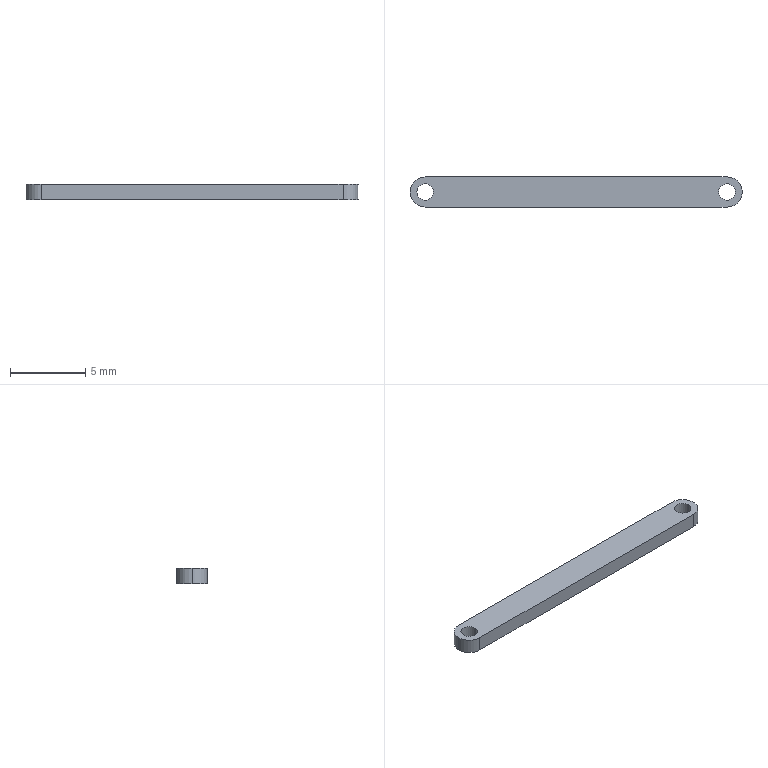Part | SolidWorks | features Extrusion 1, ICE 1 | 1 solid | 11 faces | box 22 x 2 x 1 mm | volume 41.241 mm3 | cylinder 7 | plane 4 | commonest cylinder face diameters 1.1 x4 2 x3
STEP:
#1=CARTESIAN_POINT('',(9.45,0.,0.5));
#2=VERTEX_POINT('',#1);
#3=CARTESIAN_POINT('',(10.55,0.,0.5));
#4=VERTEX_POINT('',#3);
#5=CARTESIAN_POINT('',(10.,0.,0.5));
#6=DIRECTION('',(0.,0.,1.));
#7=DIRECTION('',(1.,0.,0.));
#8=AXIS2_PLACEMENT_3D('',#5,#6,#7);
#9=CIRCLE('',#8,0.55);
#10=EDGE_CURVE('',#2,#4,#9,.T.);
#11=ORIENTED_EDGE('',*,*,#10,.T.);
#12=CARTESIAN_POINT('',(10.55,0.,-0.5));
#13=VERTEX_POINT('',#12);
#14=CARTESIAN_POINT('',(10.55,0.,0.5));
#15=DIRECTION('',(0.,0.,-1.));
#16=VECTOR('',#15,1000.);
#17=LINE('',#14,#16);
#18=EDGE_CURVE('',#4,#13,#17,.T.);
#19=ORIENTED_EDGE('',*,*,#18,.T.);
#20=CARTESIAN_POINT('',(9.45,0.,-0.5));
#21=VERTEX_POINT('',#20);
#22=CARTESIAN_POINT('',(10.,0.,-0.5));
#23=DIRECTION('',(0.,0.,1.));
#24=DIRECTION('',(1.,0.,0.));
#25=AXIS2_PLACEMENT_3D('',#22,#23,#24);
#26=CIRCLE('',#25,0.55);
#27=EDGE_CURVE('',#21,#13,#26,.T.);
#28=ORIENTED_EDGE('',*,*,#27,.F.);
#29=CARTESIAN_POINT('',(9.45,0.,0.5));
#30=DIRECTION('',(0.,0.,-1.));
#31=VECTOR('',#30,1000.);
#32=LINE('',#29,#31);
#33=EDGE_CURVE('',#2,#21,#32,.T.);
#34=ORIENTED_EDGE('',*,*,#33,.F.);
#35=EDGE_LOOP('',(#11,#19,#28,#34));
#36=FACE_OUTER_BOUND('',#35,.T.);
#37=CARTESIAN_POINT('',(10.,0.,0.5));
#38=DIRECTION('',(0.,0.,-1.));
#39=DIRECTION('',(-1.,0.,0.));
#40=AXIS2_PLACEMENT_3D('',#37,#38,#39);
#41=CYLINDRICAL_SURFACE('',#40,0.55);
#42=ADVANCED_FACE('',(#36),#41,.F.);
#43=CARTESIAN_POINT('',(-10.55,0.,0.5));
#44=VERTEX_POINT('',#43);
#45=CARTESIAN_POINT('',(-9.45,0.,0.5));
#46=VERTEX_POINT('',#45);
#47=CARTESIAN_POINT('',(-10.,0.,0.5));
#48=DIRECTION('',(0.,0.,1.));
#49=DIRECTION('',(1.,0.,0.));
#50=AXIS2_PLACEMENT_3D('',#47,#48,#49);
#51=CIRCLE('',#50,0.55);
#52=EDGE_CURVE('',#44,#46,#51,.T.);
#53=ORIENTED_EDGE('',*,*,#52,.T.);
#54=CARTESIAN_POINT('',(-9.45,0.,-0.5));
#55=VERTEX_POINT('',#54);
#56=CARTESIAN_POINT('',(-9.45,0.,0.5));
#57=DIRECTION('',(0.,0.,-1.));
#58=VECTOR('',#57,1000.);
#59=LINE('',#56,#58);
#60=EDGE_CURVE('',#46,#55,#59,.T.);
#61=ORIENTED_EDGE('',*,*,#60,.T.);
#62=CARTESIAN_POINT('',(-10.55,0.,-0.5));
#63=VERTEX_POINT('',#62);
#64=CARTESIAN_POINT('',(-10.,0.,-0.5));
#65=DIRECTION('',(0.,0.,1.));
#66=DIRECTION('',(1.,0.,0.));
#67=AXIS2_PLACEMENT_3D('',#64,#65,#66);
#68=CIRCLE('',#67,0.55);
#69=EDGE_CURVE('',#63,#55,#68,.T.);
#70=ORIENTED_EDGE('',*,*,#69,.F.);
#71=CARTESIAN_POINT('',(-10.55,0.,0.5));
#72=DIRECTION('',(0.,0.,-1.));
#73=VECTOR('',#72,1000.);
#74=LINE('',#71,#73);
#75=EDGE_CURVE('',#44,#63,#74,.T.);
#76=ORIENTED_EDGE('',*,*,#75,.F.);
#77=EDGE_LOOP('',(#53,#61,#70,#76));
#78=FACE_OUTER_BOUND('',#77,.T.);
#79=CARTESIAN_POINT('',(-10.,0.,0.5));
#80=DIRECTION('',(0.,0.,-1.));
#81=DIRECTION('',(-1.,0.,0.));
#82=AXIS2_PLACEMENT_3D('',#79,#80,#81);
#83=CYLINDRICAL_SURFACE('',#82,0.55);
#84=ADVANCED_FACE('',(#78),#83,.F.);
#85=CARTESIAN_POINT('',(-11.,0.,0.5));
#86=VERTEX_POINT('',#85);
#87=CARTESIAN_POINT('',(-10.,-1.,0.5));
#88=VERTEX_POINT('',#87);
#89=CARTESIAN_POINT('',(-10.,0.,0.5));
#90=DIRECTION('',(0.,0.,1.));
#91=DIRECTION('',(1.,0.,0.));
#92=AXIS2_PLACEMENT_3D('',#89,#90,#91);
#93=CIRCLE('',#92,1.);
#94=EDGE_CURVE('',#86,#88,#93,.T.);
#95=ORIENTED_EDGE('',*,*,#94,.F.);
#96=CARTESIAN_POINT('',(-11.,0.,-0.5));
#97=VERTEX_POINT('',#96);
#98=CARTESIAN_POINT('',(-11.,0.,0.5));
#99=DIRECTION('',(0.,0.,-1.));
#100=VECTOR('',#99,1000.);
#101=LINE('',#98,#100);
#102=EDGE_CURVE('',#86,#97,#101,.T.);
#103=ORIENTED_EDGE('',*,*,#102,.T.);
#104=CARTESIAN_POINT('',(-10.,-1.,-0.5));
#105=VERTEX_POINT('',#104);
#106=CARTESIAN_POINT('',(-10.,0.,-0.5));
#107=DIRECTION('',(0.,0.,1.));
#108=DIRECTION('',(1.,0.,0.));
#109=AXIS2_PLACEMENT_3D('',#106,#107,#108);
#110=CIRCLE('',#109,1.);
#111=EDGE_CURVE('',#97,#105,#110,.T.);
#112=ORIENTED_EDGE('',*,*,#111,.T.);
#113=CARTESIAN_POINT('',(-10.,-1.,0.5));
#114=DIRECTION('',(0.,0.,-1.));
#115=VECTOR('',#114,1000.);
#116=LINE('',#113,#115);
#117=EDGE_CURVE('',#88,#105,#116,.T.);
#118=ORIENTED_EDGE('',*,*,#117,.F.);
#119=EDGE_LOOP('',(#95,#103,#112,#118));
#120=FACE_OUTER_BOUND('',#119,.T.);
#121=CARTESIAN_POINT('',(-10.,0.,0.5));
#122=DIRECTION('',(0.,0.,-1.));
#123=DIRECTION('',(-1.,0.,0.));
#124=AXIS2_PLACEMENT_3D('',#121,#122,#123);
#125=CYLINDRICAL_SURFACE('',#124,1.);
#126=ADVANCED_FACE('',(#120),#125,.T.);
#127=ORIENTED_EDGE('',*,*,#52,.F.);
#128=CARTESIAN_POINT('',(-10.,0.,0.5));
#129=DIRECTION('',(0.,0.,1.));
#130=DIRECTION('',(1.,0.,0.));
#131=AXIS2_PLACEMENT_3D('',#128,#129,#130);
#132=CIRCLE('',#131,0.55);
#133=EDGE_CURVE('',#46,#44,#132,.T.);
#134=ORIENTED_EDGE('',*,*,#133,.F.);
#135=EDGE_LOOP('',(#127,#134));
#136=FACE_BOUND('',#135,.T.);
#137=CARTESIAN_POINT('',(-10.,1.,0.5));
#138=VERTEX_POINT('',#137);
#139=CARTESIAN_POINT('',(-10.,0.,0.5));
#140=DIRECTION('',(0.,0.,1.));
#141=DIRECTION('',(1.,0.,0.));
#142=AXIS2_PLACEMENT_3D('',#139,#140,#141);
#143=CIRCLE('',#142,1.);
#144=EDGE_CURVE('',#138,#86,#143,.T.);
#145=ORIENTED_EDGE('',*,*,#144,.T.);
#146=ORIENTED_EDGE('',*,*,#94,.T.);
#147=CARTESIAN_POINT('',(10.,-1.,0.5));
#148=VERTEX_POINT('',#147);
#149=CARTESIAN_POINT('',(-10.,-1.,0.5));
#150=DIRECTION('',(1.,0.,0.));
#151=VECTOR('',#150,1000.);
#152=LINE('',#149,#151);
#153=EDGE_CURVE('',#88,#148,#152,.T.);
#154=ORIENTED_EDGE('',*,*,#153,.T.);
#155=CARTESIAN_POINT('',(10.,1.,0.5));
#156=VERTEX_POINT('',#155);
#157=CARTESIAN_POINT('',(10.,0.,0.5));
#158=DIRECTION('',(0.,0.,1.));
#159=DIRECTION('',(1.,0.,0.));
#160=AXIS2_PLACEMENT_3D('',#157,#158,#159);
#161=CIRCLE('',#160,1.);
#162=EDGE_CURVE('',#148,#156,#161,.T.);
#163=ORIENTED_EDGE('',*,*,#162,.T.);
#164=CARTESIAN_POINT('',(-10.,1.,0.5));
#165=DIRECTION('',(-1.,0.,0.));
#166=VECTOR('',#165,1000.);
#167=LINE('',#164,#166);
#168=EDGE_CURVE('',#156,#138,#167,.T.);
#169=ORIENTED_EDGE('',*,*,#168,.T.);
#170=EDGE_LOOP('',(#145,#146,#154,#163,#169));
#171=FACE_OUTER_BOUND('',#170,.T.);
#172=ORIENTED_EDGE('',*,*,#10,.F.);
#173=CARTESIAN_POINT('',(10.,0.,0.5));
#174=DIRECTION('',(0.,0.,1.));
#175=DIRECTION('',(1.,0.,0.));
#176=AXIS2_PLACEMENT_3D('',#173,#174,#175);
#177=CIRCLE('',#176,0.55);
#178=EDGE_CURVE('',#4,#2,#177,.T.);
#179=ORIENTED_EDGE('',*,*,#178,.F.);
#180=EDGE_LOOP('',(#172,#179));
#181=FACE_BOUND('',#180,.T.);
#182=CARTESIAN_POINT('',(-10.,0.,0.5));
#183=DIRECTION('',(0.,0.,1.));
#184=DIRECTION('',(1.,0.,0.));
#185=AXIS2_PLACEMENT_3D('',#182,#183,#184);
#186=PLANE('',#185);
#187=ADVANCED_FACE('',(#136,#171,#181),#186,.T.);
#188=CARTESIAN_POINT('',(-10.,1.,-0.5));
#189=VERTEX_POINT('',#188);
#190=CARTESIAN_POINT('',(-10.,0.,-0.5));
#191=DIRECTION('',(0.,0.,1.));
#192=DIRECTION('',(1.,0.,0.));
#193=AXIS2_PLACEMENT_3D('',#190,#191,#192);
#194=CIRCLE('',#193,1.);
#195=EDGE_CURVE('',#189,#97,#194,.T.);
#196=ORIENTED_EDGE('',*,*,#195,.F.);
#197=CARTESIAN_POINT('',(10.,1.,-0.5));
#198=VERTEX_POINT('',#197);
#199=CARTESIAN_POINT('',(-10.,1.,-0.5));
#200=DIRECTION('',(-1.,0.,0.));
#201=VECTOR('',#200,1000.);
#202=LINE('',#199,#201);
#203=EDGE_CURVE('',#198,#189,#202,.T.);
#204=ORIENTED_EDGE('',*,*,#203,.F.);
#205=CARTESIAN_POINT('',(10.,-1.,-0.5));
#206=VERTEX_POINT('',#205);
#207=CARTESIAN_POINT('',(10.,0.,-0.5));
#208=DIRECTION('',(0.,0.,1.));
#209=DIRECTION('',(1.,0.,0.));
#210=AXIS2_PLACEMENT_3D('',#207,#208,#209);
#211=CIRCLE('',#210,1.);
#212=EDGE_CURVE('',#206,#198,#211,.T.);
#213=ORIENTED_EDGE('',*,*,#212,.F.);
#214=CARTESIAN_POINT('',(-10.,-1.,-0.5));
#215=DIRECTION('',(1.,0.,0.));
#216=VECTOR('',#215,1000.);
#217=LINE('',#214,#216);
#218=EDGE_CURVE('',#105,#206,#217,.T.);
#219=ORIENTED_EDGE('',*,*,#218,.F.);
#220=ORIENTED_EDGE('',*,*,#111,.F.);
#221=EDGE_LOOP('',(#196,#204,#213,#219,#220));
#222=FACE_OUTER_BOUND('',#221,.T.);
#223=ORIENTED_EDGE('',*,*,#69,.T.);
#224=CARTESIAN_POINT('',(-10.,0.,-0.5));
#225=DIRECTION('',(0.,0.,1.));
#226=DIRECTION('',(1.,0.,0.));
#227=AXIS2_PLACEMENT_3D('',#224,#225,#226);
#228=CIRCLE('',#227,0.55);
#229=EDGE_CURVE('',#55,#63,#228,.T.);
#230=ORIENTED_EDGE('',*,*,#229,.T.);
#231=EDGE_LOOP('',(#223,#230));
#232=FACE_BOUND('',#231,.T.);
#233=ORIENTED_EDGE('',*,*,#27,.T.);
#234=CARTESIAN_POINT('',(10.,0.,-0.5));
#235=DIRECTION('',(0.,0.,1.));
#236=DIRECTION('',(1.,0.,0.));
#237=AXIS2_PLACEMENT_3D('',#234,#235,#236);
#238=CIRCLE('',#237,0.55);
#239=EDGE_CURVE('',#13,#21,#238,.T.);
#240=ORIENTED_EDGE('',*,*,#239,.T.);
#241=EDGE_LOOP('',(#233,#240));
#242=FACE_BOUND('',#241,.T.);
#243=CARTESIAN_POINT('',(-10.,0.,-0.5));
#244=DIRECTION('',(0.,0.,1.));
#245=DIRECTION('',(1.,0.,0.));
#246=AXIS2_PLACEMENT_3D('',#243,#244,#245);
#247=PLANE('',#246);
#248=ADVANCED_FACE('',(#222,#232,#242),#247,.F.);
#249=ORIENTED_EDGE('',*,*,#102,.F.);
#250=ORIENTED_EDGE('',*,*,#144,.F.);
#251=CARTESIAN_POINT('',(-10.,1.,0.5));
#252=DIRECTION('',(0.,0.,-1.));
#253=VECTOR('',#252,1000.);
#254=LINE('',#251,#253);
#255=EDGE_CURVE('',#138,#189,#254,.T.);
#256=ORIENTED_EDGE('',*,*,#255,.T.);
#257=ORIENTED_EDGE('',*,*,#195,.T.);
#258=EDGE_LOOP('',(#249,#250,#256,#257));
#259=FACE_OUTER_BOUND('',#258,.T.);
#260=CARTESIAN_POINT('',(-10.,0.,0.5));
#261=DIRECTION('',(0.,0.,-1.));
#262=DIRECTION('',(-1.,0.,0.));
#263=AXIS2_PLACEMENT_3D('',#260,#261,#262);
#264=CYLINDRICAL_SURFACE('',#263,1.);
#265=ADVANCED_FACE('',(#259),#264,.T.);
#266=ORIENTED_EDGE('',*,*,#218,.T.);
#267=CARTESIAN_POINT('',(10.,-1.,0.5));
#268=DIRECTION('',(0.,0.,-1.));
#269=VECTOR('',#268,1000.);
#270=LINE('',#267,#269);
#271=EDGE_CURVE('',#148,#206,#270,.T.);
#272=ORIENTED_EDGE('',*,*,#271,.F.);
#273=ORIENTED_EDGE('',*,*,#153,.F.);
#274=ORIENTED_EDGE('',*,*,#117,.T.);
#275=EDGE_LOOP('',(#266,#272,#273,#274));
#276=FACE_OUTER_BOUND('',#275,.T.);
#277=CARTESIAN_POINT('',(-10.,-1.,0.5));
#278=DIRECTION('',(0.,1.,0.));
#279=DIRECTION('',(-1.,0.,0.));
#280=AXIS2_PLACEMENT_3D('',#277,#278,#279);
#281=PLANE('',#280);
#282=ADVANCED_FACE('',(#276),#281,.F.);
#283=ORIENTED_EDGE('',*,*,#212,.T.);
#284=CARTESIAN_POINT('',(10.,1.,0.5));
#285=DIRECTION('',(0.,0.,-1.));
#286=VECTOR('',#285,1000.);
#287=LINE('',#284,#286);
#288=EDGE_CURVE('',#156,#198,#287,.T.);
#289=ORIENTED_EDGE('',*,*,#288,.F.);
#290=ORIENTED_EDGE('',*,*,#162,.F.);
#291=ORIENTED_EDGE('',*,*,#271,.T.);
#292=EDGE_LOOP('',(#283,#289,#290,#291));
#293=FACE_OUTER_BOUND('',#292,.T.);
#294=CARTESIAN_POINT('',(10.,0.,0.5));
#295=DIRECTION('',(0.,0.,-1.));
#296=DIRECTION('',(-1.,0.,0.));
#297=AXIS2_PLACEMENT_3D('',#294,#295,#296);
#298=CYLINDRICAL_SURFACE('',#297,1.);
#299=ADVANCED_FACE('',(#293),#298,.T.);
#300=ORIENTED_EDGE('',*,*,#203,.T.);
#301=ORIENTED_EDGE('',*,*,#255,.F.);
#302=ORIENTED_EDGE('',*,*,#168,.F.);
#303=ORIENTED_EDGE('',*,*,#288,.T.);
#304=EDGE_LOOP('',(#300,#301,#302,#303));
#305=FACE_OUTER_BOUND('',#304,.T.);
#306=CARTESIAN_POINT('',(-10.,1.,0.5));
#307=DIRECTION('',(0.,-1.,0.));
#308=DIRECTION('',(1.,0.,0.));
#309=AXIS2_PLACEMENT_3D('',#306,#307,#308);
#310=PLANE('',#309);
#311=ADVANCED_FACE('',(#305),#310,.F.);
#312=ORIENTED_EDGE('',*,*,#60,.F.);
#313=ORIENTED_EDGE('',*,*,#133,.T.);
#314=ORIENTED_EDGE('',*,*,#75,.T.);
#315=ORIENTED_EDGE('',*,*,#229,.F.);
#316=EDGE_LOOP('',(#312,#313,#314,#315));
#317=FACE_OUTER_BOUND('',#316,.T.);
#318=CARTESIAN_POINT('',(-10.,0.,0.5));
#319=DIRECTION('',(0.,0.,-1.));
#320=DIRECTION('',(-1.,0.,0.));
#321=AXIS2_PLACEMENT_3D('',#318,#319,#320);
#322=CYLINDRICAL_SURFACE('',#321,0.55);
#323=ADVANCED_FACE('',(#317),#322,.F.);
#324=ORIENTED_EDGE('',*,*,#18,.F.);
#325=ORIENTED_EDGE('',*,*,#178,.T.);
#326=ORIENTED_EDGE('',*,*,#33,.T.);
#327=ORIENTED_EDGE('',*,*,#239,.F.);
#328=EDGE_LOOP('',(#324,#325,#326,#327));
#329=FACE_OUTER_BOUND('',#328,.T.);
#330=CARTESIAN_POINT('',(10.,0.,0.5));
#331=DIRECTION('',(0.,0.,-1.));
#332=DIRECTION('',(-1.,0.,0.));
#333=AXIS2_PLACEMENT_3D('',#330,#331,#332);
#334=CYLINDRICAL_SURFACE('',#333,0.55);
#335=ADVANCED_FACE('',(#329),#334,.F.);
#336=CLOSED_SHELL('',(#42,#84,#126,#187,#248,#265,#282,#299,#311,#323,#335));
#337=MANIFOLD_SOLID_BREP('',#336);
#338=CARTESIAN_POINT('',(0.,0.,0.));
#339=DIRECTION('',(0.,0.,1.));
#340=DIRECTION('',(1.,0.,0.));
#341=AXIS2_PLACEMENT_3D('',#338,#339,#340);
#342=(LENGTH_UNIT()NAMED_UNIT(*)SI_UNIT(.MILLI.,.METRE.));
#343=UNCERTAINTY_MEASURE_WITH_UNIT(LENGTH_MEASURE(0.00001),#342,'','');
#344=(NAMED_UNIT(*)PLANE_ANGLE_UNIT()SI_UNIT($,.RADIAN.));
#345=(NAMED_UNIT(*)SI_UNIT($,.STERADIAN.)SOLID_ANGLE_UNIT());
#346=(GEOMETRIC_REPRESENTATION_CONTEXT(3)GLOBAL_UNCERTAINTY_ASSIGNED_CONTEXT((#343))GLOBAL_UNIT_ASSIGNED_CONTEXT((#342,#344,#345))REPRESENTATION_CONTEXT('',''));
#347=ADVANCED_BREP_SHAPE_REPRESENTATION('',(#337,#341),#346);